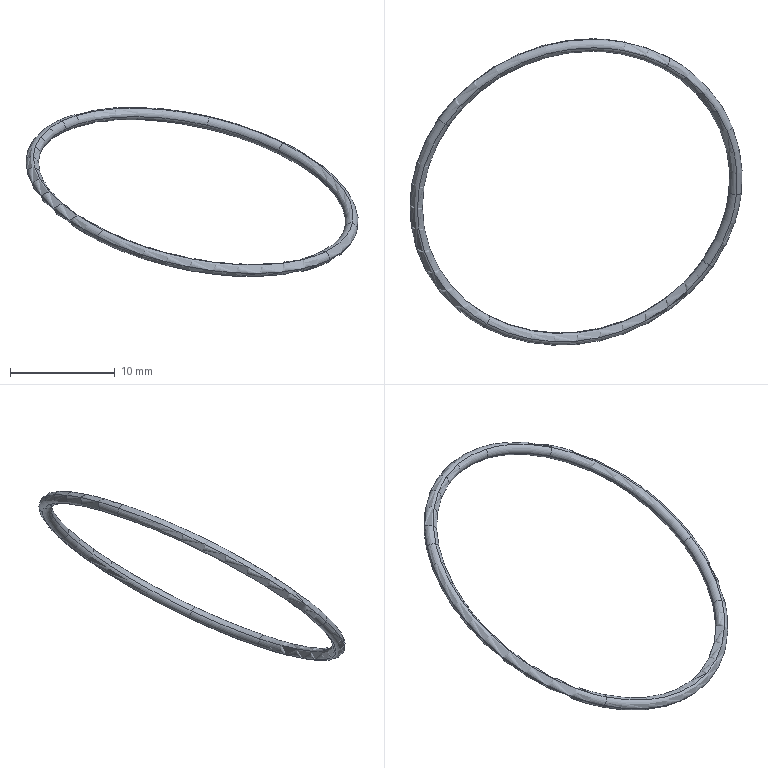Part | SolidWorks | features BaseBody 1 | 1 solid | 22 faces | box 31.731 x 29.251 x 16.171 mm | volume 110.749 mm3 | torus 22
STEP:
#1=CARTESIAN_POINT('',(1961.202,-199.266,900.389));
#2=VERTEX_POINT('',#1);
#3=CARTESIAN_POINT('',(1954.63,-186.958,908.017));
#4=VERTEX_POINT('',#3);
#5=CARTESIAN_POINT('',(1961.202,-199.266,900.389));
#6=CARTESIAN_POINT('',(1961.789,-193.856,902.943));
#7=CARTESIAN_POINT('',(1959.22,-189.407,905.745));
#8=CARTESIAN_POINT('',(1954.63,-186.958,908.017));
#9=(BOUNDED_CURVE()B_SPLINE_CURVE(3,(#5,#6,#7,#8),.UNSPECIFIED.,.F.,.F.)B_SPLINE_CURVE_WITH_KNOTS((4,4),(0.3237,1.),.UNSPECIFIED.)CURVE()GEOMETRIC_REPRESENTATION_ITEM()RATIONAL_B_SPLINE_CURVE((1.167,1.112,1.178,1.363))REPRESENTATION_ITEM(''));
#10=EDGE_CURVE('',#2,#4,#9,.T.);
#11=ORIENTED_EDGE('',*,*,#10,.F.);
#12=CARTESIAN_POINT('',(1960.738,-199.528,901.049));
#13=VERTEX_POINT('',#12);
#14=CARTESIAN_POINT('',(1961.323,-199.528,900.915));
#15=DIRECTION('',(0.09761,0.8999,0.425));
#16=DIRECTION('',(0.,-0.427,0.9043));
#17=AXIS2_PLACEMENT_3D('',#14,#15,#16);
#18=CIRCLE('',#17,0.6);
#19=EDGE_CURVE('',#2,#13,#18,.T.);
#20=ORIENTED_EDGE('',*,*,#19,.T.);
#21=CARTESIAN_POINT('',(1954.419,-187.693,908.384));
#22=VERTEX_POINT('',#21);
#23=CARTESIAN_POINT('',(1960.738,-199.528,901.049));
#24=CARTESIAN_POINT('',(1961.302,-194.326,903.505));
#25=CARTESIAN_POINT('',(1958.832,-190.049,906.199));
#26=CARTESIAN_POINT('',(1954.419,-187.693,908.384));
#27=(BOUNDED_CURVE()B_SPLINE_CURVE(3,(#23,#24,#25,#26),.UNSPECIFIED.,.F.,.F.)B_SPLINE_CURVE_WITH_KNOTS((4,4),(0.3237,1.),.UNSPECIFIED.)CURVE()GEOMETRIC_REPRESENTATION_ITEM()RATIONAL_B_SPLINE_CURVE((1.216,1.159,1.228,1.421))REPRESENTATION_ITEM(''));
#28=EDGE_CURVE('',#13,#22,#27,.T.);
#29=ORIENTED_EDGE('',*,*,#28,.T.);
#30=CARTESIAN_POINT('',(1954.63,-186.958,908.017));
#31=CARTESIAN_POINT('',(1954.434,-187.238,907.923));
#32=CARTESIAN_POINT('',(1954.349,-187.541,908.078));
#33=CARTESIAN_POINT('',(1954.419,-187.693,908.384));
#34=(BOUNDED_CURVE()B_SPLINE_CURVE(3,(#30,#31,#32,#33),.UNSPECIFIED.,.F.,.T.)B_SPLINE_CURVE_WITH_KNOTS((4,4),(0.,1.),.UNSPECIFIED.)CURVE()GEOMETRIC_REPRESENTATION_ITEM()RATIONAL_B_SPLINE_CURVE((1.363,1.111,1.13,1.421))REPRESENTATION_ITEM(''));
#35=EDGE_CURVE('',#4,#22,#34,.T.);
#36=ORIENTED_EDGE('',*,*,#35,.F.);
#37=EDGE_LOOP('',(#11,#20,#29,#36));
#38=FACE_OUTER_BOUND('',#37,.T.);
#39=CARTESIAN_POINT('',(1946.133,-199.528,904.404));
#40=DIRECTION('',(-0.2015,0.436,-0.8771));
#41=DIRECTION('',(0.9746,0.,-0.2239));
#42=AXIS2_PLACEMENT_3D('',#39,#40,#41);
#43=TOROIDAL_SURFACE('',#42,15.585,0.6);
#44=ADVANCED_FACE('',(#38),#43,.T.);
#45=CARTESIAN_POINT('',(1947.596,-186.042,910.772));
#46=VERTEX_POINT('',#45);
#47=CARTESIAN_POINT('',(1934.018,-193.063,910.401));
#48=VERTEX_POINT('',#47);
#49=CARTESIAN_POINT('',(1947.596,-186.042,910.772));
#50=CARTESIAN_POINT('',(1941.997,-186.042,912.058));
#51=CARTESIAN_POINT('',(1937.057,-188.722,911.86));
#52=CARTESIAN_POINT('',(1934.018,-193.063,910.401));
#53=(BOUNDED_CURVE()B_SPLINE_CURVE(3,(#49,#50,#51,#52),.UNSPECIFIED.,.F.,.T.)B_SPLINE_CURVE_WITH_KNOTS((4,4),(0.3294,1.),.UNSPECIFIED.)CURVE()GEOMETRIC_REPRESENTATION_ITEM()RATIONAL_B_SPLINE_CURVE((1.228,1.157,1.209,1.385))REPRESENTATION_ITEM(''));
#54=EDGE_CURVE('',#46,#48,#53,.T.);
#55=ORIENTED_EDGE('',*,*,#54,.F.);
#56=CARTESIAN_POINT('',(1947.776,-185.764,911.553));
#57=VERTEX_POINT('',#56);
#58=CARTESIAN_POINT('',(1947.655,-185.502,911.027));
#59=DIRECTION('',(-0.9746,0.,0.2239));
#60=DIRECTION('',(0.2239,0.,0.9746));
#61=AXIS2_PLACEMENT_3D('',#58,#59,#60);
#62=CIRCLE('',#61,0.6);
#63=EDGE_CURVE('',#46,#57,#62,.T.);
#64=ORIENTED_EDGE('',*,*,#63,.T.);
#65=CARTESIAN_POINT('',(1933.654,-193.065,911.167));
#66=VERTEX_POINT('',#65);
#67=CARTESIAN_POINT('',(1947.776,-185.764,911.553));
#68=CARTESIAN_POINT('',(1941.953,-185.764,912.89));
#69=CARTESIAN_POINT('',(1936.814,-188.551,912.685));
#70=CARTESIAN_POINT('',(1933.654,-193.065,911.167));
#71=(BOUNDED_CURVE()B_SPLINE_CURVE(3,(#67,#68,#69,#70),.UNSPECIFIED.,.F.,.F.)B_SPLINE_CURVE_WITH_KNOTS((4,4),(0.3294,1.),.UNSPECIFIED.)CURVE()GEOMETRIC_REPRESENTATION_ITEM()RATIONAL_B_SPLINE_CURVE((1.178,1.11,1.16,1.328))REPRESENTATION_ITEM(''));
#72=EDGE_CURVE('',#57,#66,#71,.T.);
#73=ORIENTED_EDGE('',*,*,#72,.T.);
#74=CARTESIAN_POINT('',(1934.018,-193.063,910.401));
#75=CARTESIAN_POINT('',(1934.088,-193.215,910.706));
#76=CARTESIAN_POINT('',(1933.94,-193.218,911.025));
#77=CARTESIAN_POINT('',(1933.654,-193.065,911.167));
#78=(BOUNDED_CURVE()B_SPLINE_CURVE(3,(#74,#75,#76,#77),.UNSPECIFIED.,.F.,.F.)B_SPLINE_CURVE_WITH_KNOTS((4,4),(0.,1.),.UNSPECIFIED.)CURVE()GEOMETRIC_REPRESENTATION_ITEM()RATIONAL_B_SPLINE_CURVE((1.385,1.101,1.082,1.328))REPRESENTATION_ITEM(''));
#79=EDGE_CURVE('',#48,#66,#78,.T.);
#80=ORIENTED_EDGE('',*,*,#79,.F.);
#81=EDGE_LOOP('',(#55,#64,#73,#80));
#82=FACE_OUTER_BOUND('',#81,.T.);
#83=CARTESIAN_POINT('',(1946.133,-199.528,904.404));
#84=DIRECTION('',(-0.2015,0.436,-0.8771));
#85=DIRECTION('',(0.09761,0.8999,0.425));
#86=AXIS2_PLACEMENT_3D('',#83,#84,#85);
#87=TOROIDAL_SURFACE('',#86,15.585,0.6);
#88=ADVANCED_FACE('',(#82),#87,.T.);
#89=CARTESIAN_POINT('',(1947.713,-184.963,911.282));
#90=VERTEX_POINT('',#89);
#91=CARTESIAN_POINT('',(1933.048,-192.545,910.881));
#92=VERTEX_POINT('',#91);
#93=CARTESIAN_POINT('',(1947.713,-184.963,911.282));
#94=CARTESIAN_POINT('',(1941.666,-184.963,912.671));
#95=CARTESIAN_POINT('',(1936.33,-187.857,912.457));
#96=CARTESIAN_POINT('',(1933.048,-192.545,910.881));
#97=(BOUNDED_CURVE()B_SPLINE_CURVE(3,(#93,#94,#95,#96),.UNSPECIFIED.,.F.,.F.)B_SPLINE_CURVE_WITH_KNOTS((4,4),(0.3294,1.),.UNSPECIFIED.)CURVE()GEOMETRIC_REPRESENTATION_ITEM()RATIONAL_B_SPLINE_CURVE((1.228,1.157,1.209,1.385))REPRESENTATION_ITEM(''));
#98=EDGE_CURVE('',#90,#92,#97,.T.);
#99=ORIENTED_EDGE('',*,*,#98,.F.);
#100=CARTESIAN_POINT('',(1947.534,-185.241,910.5));
#101=VERTEX_POINT('',#100);
#102=CARTESIAN_POINT('',(1947.655,-185.502,911.027));
#103=DIRECTION('',(-0.9746,0.,0.2239));
#104=DIRECTION('',(0.2239,0.,0.9746));
#105=AXIS2_PLACEMENT_3D('',#102,#103,#104);
#106=CIRCLE('',#105,0.6);
#107=EDGE_CURVE('',#90,#101,#106,.T.);
#108=ORIENTED_EDGE('',*,*,#107,.T.);
#109=CARTESIAN_POINT('',(1933.412,-192.542,910.115));
#110=VERTEX_POINT('',#109);
#111=CARTESIAN_POINT('',(1947.534,-185.241,910.5));
#112=CARTESIAN_POINT('',(1941.711,-185.241,911.838));
#113=CARTESIAN_POINT('',(1936.572,-188.028,911.633));
#114=CARTESIAN_POINT('',(1933.412,-192.542,910.115));
#115=(BOUNDED_CURVE()B_SPLINE_CURVE(3,(#111,#112,#113,#114),.UNSPECIFIED.,.F.,.F.)B_SPLINE_CURVE_WITH_KNOTS((4,4),(0.3294,1.),.UNSPECIFIED.)CURVE()GEOMETRIC_REPRESENTATION_ITEM()RATIONAL_B_SPLINE_CURVE((1.178,1.11,1.16,1.328))REPRESENTATION_ITEM(''));
#116=EDGE_CURVE('',#101,#110,#115,.T.);
#117=ORIENTED_EDGE('',*,*,#116,.T.);
#118=CARTESIAN_POINT('',(1933.048,-192.545,910.881));
#119=CARTESIAN_POINT('',(1932.977,-192.393,910.575));
#120=CARTESIAN_POINT('',(1933.125,-192.389,910.256));
#121=CARTESIAN_POINT('',(1933.412,-192.542,910.115));
#122=(BOUNDED_CURVE()B_SPLINE_CURVE(3,(#118,#119,#120,#121),.UNSPECIFIED.,.F.,.F.)B_SPLINE_CURVE_WITH_KNOTS((4,4),(0.,1.),.UNSPECIFIED.)CURVE()GEOMETRIC_REPRESENTATION_ITEM()RATIONAL_B_SPLINE_CURVE((1.385,1.101,1.082,1.328))REPRESENTATION_ITEM(''));
#123=EDGE_CURVE('',#92,#110,#122,.T.);
#124=ORIENTED_EDGE('',*,*,#123,.F.);
#125=EDGE_LOOP('',(#99,#108,#117,#124));
#126=FACE_OUTER_BOUND('',#125,.T.);
#127=CARTESIAN_POINT('',(1946.133,-199.528,904.404));
#128=DIRECTION('',(-0.2015,0.436,-0.8771));
#129=DIRECTION('',(0.09761,0.8999,0.425));
#130=AXIS2_PLACEMENT_3D('',#127,#128,#129);
#131=TOROIDAL_SURFACE('',#130,15.585,0.6);
#132=ADVANCED_FACE('',(#126),#131,.T.);
#133=ORIENTED_EDGE('',*,*,#28,.F.);
#134=CARTESIAN_POINT('',(1961.444,-199.79,901.441));
#135=VERTEX_POINT('',#134);
#136=CARTESIAN_POINT('',(1961.323,-199.528,900.915));
#137=DIRECTION('',(0.09761,0.8999,0.425));
#138=DIRECTION('',(0.,-0.427,0.9043));
#139=AXIS2_PLACEMENT_3D('',#136,#137,#138);
#140=CIRCLE('',#139,0.6);
#141=EDGE_CURVE('',#13,#135,#140,.T.);
#142=ORIENTED_EDGE('',*,*,#141,.T.);
#143=CARTESIAN_POINT('',(1954.871,-187.481,909.069));
#144=VERTEX_POINT('',#143);
#145=CARTESIAN_POINT('',(1961.444,-199.79,901.441));
#146=CARTESIAN_POINT('',(1962.03,-194.38,903.996));
#147=CARTESIAN_POINT('',(1959.462,-189.931,906.797));
#148=CARTESIAN_POINT('',(1954.871,-187.481,909.069));
#149=(BOUNDED_CURVE()B_SPLINE_CURVE(3,(#145,#146,#147,#148),.UNSPECIFIED.,.F.,.F.)B_SPLINE_CURVE_WITH_KNOTS((4,4),(0.3237,1.),.UNSPECIFIED.)CURVE()GEOMETRIC_REPRESENTATION_ITEM()RATIONAL_B_SPLINE_CURVE((1.167,1.112,1.178,1.363))REPRESENTATION_ITEM(''));
#150=EDGE_CURVE('',#135,#144,#149,.T.);
#151=ORIENTED_EDGE('',*,*,#150,.T.);
#152=CARTESIAN_POINT('',(1954.419,-187.693,908.384));
#153=CARTESIAN_POINT('',(1954.489,-187.845,908.689));
#154=CARTESIAN_POINT('',(1954.675,-187.761,908.975));
#155=CARTESIAN_POINT('',(1954.871,-187.481,909.069));
#156=(BOUNDED_CURVE()B_SPLINE_CURVE(3,(#152,#153,#154,#155),.UNSPECIFIED.,.F.,.F.)B_SPLINE_CURVE_WITH_KNOTS((4,4),(0.,1.),.UNSPECIFIED.)CURVE()GEOMETRIC_REPRESENTATION_ITEM()RATIONAL_B_SPLINE_CURVE((1.421,1.13,1.111,1.363))REPRESENTATION_ITEM(''));
#157=EDGE_CURVE('',#22,#144,#156,.T.);
#158=ORIENTED_EDGE('',*,*,#157,.F.);
#159=EDGE_LOOP('',(#133,#142,#151,#158));
#160=FACE_OUTER_BOUND('',#159,.T.);
#161=CARTESIAN_POINT('',(1946.133,-199.528,904.404));
#162=DIRECTION('',(-0.2015,0.436,-0.8771));
#163=DIRECTION('',(0.9746,0.,-0.2239));
#164=AXIS2_PLACEMENT_3D('',#161,#162,#163);
#165=TOROIDAL_SURFACE('',#164,15.585,0.6);
#166=ADVANCED_FACE('',(#160),#165,.T.);
#167=CARTESIAN_POINT('',(1961.908,-199.528,900.78));
#168=VERTEX_POINT('',#167);
#169=CARTESIAN_POINT('',(1955.082,-186.746,908.702));
#170=VERTEX_POINT('',#169);
#171=CARTESIAN_POINT('',(1961.908,-199.528,900.78));
#172=CARTESIAN_POINT('',(1962.517,-193.91,903.433));
#173=CARTESIAN_POINT('',(1959.849,-189.289,906.343));
#174=CARTESIAN_POINT('',(1955.082,-186.746,908.702));
#175=(BOUNDED_CURVE()B_SPLINE_CURVE(3,(#171,#172,#173,#174),.UNSPECIFIED.,.F.,.F.)B_SPLINE_CURVE_WITH_KNOTS((4,4),(0.3237,1.),.UNSPECIFIED.)CURVE()GEOMETRIC_REPRESENTATION_ITEM()RATIONAL_B_SPLINE_CURVE((1.216,1.159,1.228,1.421))REPRESENTATION_ITEM(''));
#176=EDGE_CURVE('',#168,#170,#175,.T.);
#177=ORIENTED_EDGE('',*,*,#176,.F.);
#178=CARTESIAN_POINT('',(1961.323,-199.528,900.915));
#179=DIRECTION('',(0.09761,0.8999,0.425));
#180=DIRECTION('',(0.,-0.427,0.9043));
#181=AXIS2_PLACEMENT_3D('',#178,#179,#180);
#182=CIRCLE('',#181,0.6);
#183=EDGE_CURVE('',#168,#2,#182,.T.);
#184=ORIENTED_EDGE('',*,*,#183,.T.);
#185=ORIENTED_EDGE('',*,*,#10,.T.);
#186=CARTESIAN_POINT('',(1955.082,-186.746,908.702));
#187=CARTESIAN_POINT('',(1955.012,-186.594,908.397));
#188=CARTESIAN_POINT('',(1954.826,-186.678,908.111));
#189=CARTESIAN_POINT('',(1954.63,-186.958,908.017));
#190=(BOUNDED_CURVE()B_SPLINE_CURVE(3,(#186,#187,#188,#189),.UNSPECIFIED.,.F.,.F.)B_SPLINE_CURVE_WITH_KNOTS((4,4),(0.,1.),.UNSPECIFIED.)CURVE()GEOMETRIC_REPRESENTATION_ITEM()RATIONAL_B_SPLINE_CURVE((1.421,1.13,1.111,1.363))REPRESENTATION_ITEM(''));
#191=EDGE_CURVE('',#170,#4,#190,.T.);
#192=ORIENTED_EDGE('',*,*,#191,.F.);
#193=EDGE_LOOP('',(#177,#184,#185,#192));
#194=FACE_OUTER_BOUND('',#193,.T.);
#195=CARTESIAN_POINT('',(1946.133,-199.528,904.404));
#196=DIRECTION('',(-0.2015,0.436,-0.8771));
#197=DIRECTION('',(0.9746,0.,-0.2239));
#198=AXIS2_PLACEMENT_3D('',#195,#196,#197);
#199=TOROIDAL_SURFACE('',#198,15.585,0.6);
#200=ADVANCED_FACE('',(#194),#199,.T.);
#201=ORIENTED_EDGE('',*,*,#150,.F.);
#202=CARTESIAN_POINT('',(1961.323,-199.528,900.915));
#203=DIRECTION('',(0.09761,0.8999,0.425));
#204=DIRECTION('',(0.,-0.427,0.9043));
#205=AXIS2_PLACEMENT_3D('',#202,#203,#204);
#206=CIRCLE('',#205,0.6);
#207=EDGE_CURVE('',#135,#168,#206,.T.);
#208=ORIENTED_EDGE('',*,*,#207,.T.);
#209=ORIENTED_EDGE('',*,*,#176,.T.);
#210=CARTESIAN_POINT('',(1954.871,-187.481,909.069));
#211=CARTESIAN_POINT('',(1955.067,-187.201,909.164));
#212=CARTESIAN_POINT('',(1955.153,-186.898,909.008));
#213=CARTESIAN_POINT('',(1955.082,-186.746,908.702));
#214=(BOUNDED_CURVE()B_SPLINE_CURVE(3,(#210,#211,#212,#213),.UNSPECIFIED.,.F.,.F.)B_SPLINE_CURVE_WITH_KNOTS((4,4),(0.,1.),.UNSPECIFIED.)CURVE()GEOMETRIC_REPRESENTATION_ITEM()RATIONAL_B_SPLINE_CURVE((1.363,1.111,1.13,1.421))REPRESENTATION_ITEM(''));
#215=EDGE_CURVE('',#144,#170,#214,.T.);
#216=ORIENTED_EDGE('',*,*,#215,.F.);
#217=EDGE_LOOP('',(#201,#208,#209,#216));
#218=FACE_OUTER_BOUND('',#217,.T.);
#219=CARTESIAN_POINT('',(1946.133,-199.528,904.404));
#220=DIRECTION('',(-0.2015,0.436,-0.8771));
#221=DIRECTION('',(0.9746,0.,-0.2239));
#222=AXIS2_PLACEMENT_3D('',#219,#220,#221);
#223=TOROIDAL_SURFACE('',#222,15.585,0.6);
#224=ADVANCED_FACE('',(#218),#223,.T.);
#225=CARTESIAN_POINT('',(1937.637,-212.098,900.791));
#226=VERTEX_POINT('',#225);
#227=CARTESIAN_POINT('',(1937.184,-212.31,900.105));
#228=VERTEX_POINT('',#227);
#229=CARTESIAN_POINT('',(1937.637,-212.098,900.791));
#230=CARTESIAN_POINT('',(1937.441,-212.378,900.696));
#231=CARTESIAN_POINT('',(1937.255,-212.462,900.411));
#232=CARTESIAN_POINT('',(1937.184,-212.31,900.105));
#233=(BOUNDED_CURVE()B_SPLINE_CURVE(3,(#229,#230,#231,#232),.UNSPECIFIED.,.F.,.F.)B_SPLINE_CURVE_WITH_KNOTS((4,4),(0.,1.),.UNSPECIFIED.)CURVE()GEOMETRIC_REPRESENTATION_ITEM()RATIONAL_B_SPLINE_CURVE((1.363,1.111,1.13,1.421))REPRESENTATION_ITEM(''));
#234=EDGE_CURVE('',#226,#228,#233,.T.);
#235=ORIENTED_EDGE('',*,*,#234,.T.);
#236=CARTESIAN_POINT('',(1959.219,-206.511,897.927));
#237=VERTEX_POINT('',#236);
#238=CARTESIAN_POINT('',(1937.184,-212.31,900.105));
#239=CARTESIAN_POINT('',(1944.808,-216.379,896.331));
#240=CARTESIAN_POINT('',(1953.949,-214.039,895.395));
#241=CARTESIAN_POINT('',(1959.219,-206.511,897.927));
#242=(BOUNDED_CURVE()B_SPLINE_CURVE(3,(#238,#239,#240,#241),.UNSPECIFIED.,.F.,.F.)B_SPLINE_CURVE_WITH_KNOTS((4,4),(0.,1.),.UNSPECIFIED.)CURVE()GEOMETRIC_REPRESENTATION_ITEM()RATIONAL_B_SPLINE_CURVE((1.421,1.135,1.123,1.385))REPRESENTATION_ITEM(''));
#243=EDGE_CURVE('',#228,#237,#242,.T.);
#244=ORIENTED_EDGE('',*,*,#243,.T.);
#245=CARTESIAN_POINT('',(1958.855,-206.514,898.693));
#246=VERTEX_POINT('',#245);
#247=CARTESIAN_POINT('',(1958.734,-206.252,898.167));
#248=DIRECTION('',(0.5529,0.7898,0.2656));
#249=DIRECTION('',(0.8085,-0.4315,-0.4002));
#250=AXIS2_PLACEMENT_3D('',#247,#248,#249);
#251=CIRCLE('',#250,0.6);
#252=EDGE_CURVE('',#246,#237,#251,.T.);
#253=ORIENTED_EDGE('',*,*,#252,.F.);
#254=CARTESIAN_POINT('',(1937.637,-212.098,900.791));
#255=CARTESIAN_POINT('',(1944.978,-216.016,897.157));
#256=CARTESIAN_POINT('',(1953.78,-213.763,896.255));
#257=CARTESIAN_POINT('',(1958.855,-206.514,898.693));
#258=(BOUNDED_CURVE()B_SPLINE_CURVE(3,(#254,#255,#256,#257),.UNSPECIFIED.,.F.,.F.)B_SPLINE_CURVE_WITH_KNOTS((4,4),(0.,1.),.UNSPECIFIED.)CURVE()GEOMETRIC_REPRESENTATION_ITEM()RATIONAL_B_SPLINE_CURVE((1.363,1.089,1.077,1.328))REPRESENTATION_ITEM(''));
#259=EDGE_CURVE('',#226,#246,#258,.T.);
#260=ORIENTED_EDGE('',*,*,#259,.F.);
#261=EDGE_LOOP('',(#235,#244,#253,#260));
#262=FACE_OUTER_BOUND('',#261,.T.);
#263=CARTESIAN_POINT('',(1946.133,-199.528,904.404));
#264=DIRECTION('',(-0.2015,0.436,-0.8771));
#265=DIRECTION('',(0.9746,0.,-0.2239));
#266=AXIS2_PLACEMENT_3D('',#263,#264,#265);
#267=TOROIDAL_SURFACE('',#266,15.585,0.6);
#268=ADVANCED_FACE('',(#262),#267,.T.);
#269=CARTESIAN_POINT('',(1933.048,-192.545,910.881));
#270=CARTESIAN_POINT('',(1927.777,-200.073,908.349));
#271=CARTESIAN_POINT('',(1929.56,-208.242,903.879));
#272=CARTESIAN_POINT('',(1937.184,-212.31,900.105));
#273=(BOUNDED_CURVE()B_SPLINE_CURVE(3,(#269,#270,#271,#272),.UNSPECIFIED.,.F.,.F.)B_SPLINE_CURVE_WITH_KNOTS((4,4),(0.,1.),.UNSPECIFIED.)CURVE()GEOMETRIC_REPRESENTATION_ITEM()RATIONAL_B_SPLINE_CURVE((1.385,1.123,1.135,1.421))REPRESENTATION_ITEM(''));
#274=EDGE_CURVE('',#92,#228,#273,.T.);
#275=ORIENTED_EDGE('',*,*,#274,.T.);
#276=ORIENTED_EDGE('',*,*,#234,.F.);
#277=CARTESIAN_POINT('',(1933.654,-193.065,911.167));
#278=CARTESIAN_POINT('',(1928.579,-200.314,908.729));
#279=CARTESIAN_POINT('',(1930.296,-208.181,904.424));
#280=CARTESIAN_POINT('',(1937.637,-212.098,900.791));
#281=(BOUNDED_CURVE()B_SPLINE_CURVE(3,(#277,#278,#279,#280),.UNSPECIFIED.,.F.,.T.)B_SPLINE_CURVE_WITH_KNOTS((4,4),(0.,1.),.UNSPECIFIED.)CURVE()GEOMETRIC_REPRESENTATION_ITEM()RATIONAL_B_SPLINE_CURVE((1.328,1.077,1.089,1.363))REPRESENTATION_ITEM(''));
#282=EDGE_CURVE('',#66,#226,#281,.T.);
#283=ORIENTED_EDGE('',*,*,#282,.F.);
#284=CARTESIAN_POINT('',(1933.654,-193.065,911.167));
#285=CARTESIAN_POINT('',(1933.367,-192.912,911.309));
#286=CARTESIAN_POINT('',(1933.118,-192.697,911.187));
#287=CARTESIAN_POINT('',(1933.048,-192.545,910.881));
#288=(BOUNDED_CURVE()B_SPLINE_CURVE(3,(#284,#285,#286,#287),.UNSPECIFIED.,.F.,.T.)B_SPLINE_CURVE_WITH_KNOTS((4,4),(0.,1.),.UNSPECIFIED.)CURVE()GEOMETRIC_REPRESENTATION_ITEM()RATIONAL_B_SPLINE_CURVE((1.328,1.082,1.101,1.385))REPRESENTATION_ITEM(''));
#289=EDGE_CURVE('',#66,#92,#288,.T.);
#290=ORIENTED_EDGE('',*,*,#289,.T.);
#291=EDGE_LOOP('',(#275,#276,#283,#290));
#292=FACE_OUTER_BOUND('',#291,.T.);
#293=CARTESIAN_POINT('',(1946.133,-199.528,904.404));
#294=DIRECTION('',(-0.2015,0.436,-0.8771));
#295=DIRECTION('',(0.9746,0.,-0.2239));
#296=AXIS2_PLACEMENT_3D('',#293,#294,#295);
#297=TOROIDAL_SURFACE('',#296,15.585,0.6);
#298=ADVANCED_FACE('',(#292),#297,.T.);
#299=ORIENTED_EDGE('',*,*,#243,.F.);
#300=CARTESIAN_POINT('',(1937.395,-211.575,899.738));
#301=VERTEX_POINT('',#300);
#302=CARTESIAN_POINT('',(1937.184,-212.31,900.105));
#303=CARTESIAN_POINT('',(1937.114,-212.159,899.799));
#304=CARTESIAN_POINT('',(1937.199,-211.855,899.644));
#305=CARTESIAN_POINT('',(1937.395,-211.575,899.738));
#306=(BOUNDED_CURVE()B_SPLINE_CURVE(3,(#302,#303,#304,#305),.UNSPECIFIED.,.F.,.F.)B_SPLINE_CURVE_WITH_KNOTS((4,4),(0.,1.),.UNSPECIFIED.)CURVE()GEOMETRIC_REPRESENTATION_ITEM()RATIONAL_B_SPLINE_CURVE((1.421,1.13,1.111,1.363))REPRESENTATION_ITEM(''));
#307=EDGE_CURVE('',#228,#301,#306,.T.);
#308=ORIENTED_EDGE('',*,*,#307,.T.);
#309=CARTESIAN_POINT('',(1958.613,-205.991,897.64));
#310=VERTEX_POINT('',#309);
#311=CARTESIAN_POINT('',(1937.395,-211.575,899.738));
#312=CARTESIAN_POINT('',(1944.737,-215.493,896.104));
#313=CARTESIAN_POINT('',(1953.538,-213.24,895.203));
#314=CARTESIAN_POINT('',(1958.613,-205.991,897.64));
#315=(BOUNDED_CURVE()B_SPLINE_CURVE(3,(#311,#312,#313,#314),.UNSPECIFIED.,.F.,.F.)B_SPLINE_CURVE_WITH_KNOTS((4,4),(0.,1.),.UNSPECIFIED.)CURVE()GEOMETRIC_REPRESENTATION_ITEM()RATIONAL_B_SPLINE_CURVE((1.363,1.089,1.077,1.328))REPRESENTATION_ITEM(''));
#316=EDGE_CURVE('',#301,#310,#315,.T.);
#317=ORIENTED_EDGE('',*,*,#316,.T.);
#318=CARTESIAN_POINT('',(1959.219,-206.511,897.927));
#319=CARTESIAN_POINT('',(1959.149,-206.359,897.621));
#320=CARTESIAN_POINT('',(1958.9,-206.144,897.499));
#321=CARTESIAN_POINT('',(1958.613,-205.991,897.64));
#322=(BOUNDED_CURVE()B_SPLINE_CURVE(3,(#318,#319,#320,#321),.UNSPECIFIED.,.F.,.F.)B_SPLINE_CURVE_WITH_KNOTS((4,4),(0.,1.),.UNSPECIFIED.)CURVE()GEOMETRIC_REPRESENTATION_ITEM()RATIONAL_B_SPLINE_CURVE((1.385,1.101,1.082,1.328))REPRESENTATION_ITEM(''));
#323=EDGE_CURVE('',#237,#310,#322,.T.);
#324=ORIENTED_EDGE('',*,*,#323,.F.);
#325=EDGE_LOOP('',(#299,#308,#317,#324));
#326=FACE_OUTER_BOUND('',#325,.T.);
#327=CARTESIAN_POINT('',(1946.133,-199.528,904.404));
#328=DIRECTION('',(-0.2015,0.436,-0.8771));
#329=DIRECTION('',(0.09761,0.8999,0.425));
#330=AXIS2_PLACEMENT_3D('',#327,#328,#329);
#331=TOROIDAL_SURFACE('',#330,15.585,0.6);
#332=ADVANCED_FACE('',(#326),#331,.T.);
#333=ORIENTED_EDGE('',*,*,#207,.F.);
#334=CARTESIAN_POINT('',(1958.855,-206.514,898.693));
#335=CARTESIAN_POINT('',(1960.274,-204.487,899.375));
#336=CARTESIAN_POINT('',(1961.182,-202.203,900.301));
#337=CARTESIAN_POINT('',(1961.444,-199.79,901.441));
#338=(BOUNDED_CURVE()B_SPLINE_CURVE(3,(#334,#335,#336,#337),.UNSPECIFIED.,.F.,.F.)B_SPLINE_CURVE_WITH_KNOTS((4,4),(0.,0.3237),.UNSPECIFIED.)CURVE()GEOMETRIC_REPRESENTATION_ITEM()RATIONAL_B_SPLINE_CURVE((1.328,1.247,1.193,1.167))REPRESENTATION_ITEM(''));
#339=EDGE_CURVE('',#246,#135,#338,.T.);
#340=ORIENTED_EDGE('',*,*,#339,.F.);
#341=ORIENTED_EDGE('',*,*,#252,.T.);
#342=CARTESIAN_POINT('',(1959.219,-206.511,897.927));
#343=CARTESIAN_POINT('',(1960.693,-204.406,898.635));
#344=CARTESIAN_POINT('',(1961.636,-202.035,899.597));
#345=CARTESIAN_POINT('',(1961.908,-199.528,900.78));
#346=(BOUNDED_CURVE()B_SPLINE_CURVE(3,(#342,#343,#344,#345),.UNSPECIFIED.,.F.,.F.)B_SPLINE_CURVE_WITH_KNOTS((4,4),(0.,0.3237),.UNSPECIFIED.)CURVE()GEOMETRIC_REPRESENTATION_ITEM()RATIONAL_B_SPLINE_CURVE((1.385,1.3,1.244,1.216))REPRESENTATION_ITEM(''));
#347=EDGE_CURVE('',#237,#168,#346,.T.);
#348=ORIENTED_EDGE('',*,*,#347,.T.);
#349=EDGE_LOOP('',(#333,#340,#341,#348));
#350=FACE_OUTER_BOUND('',#349,.T.);
#351=CARTESIAN_POINT('',(1946.133,-199.528,904.404));
#352=DIRECTION('',(-0.2015,0.436,-0.8771));
#353=DIRECTION('',(0.9746,0.,-0.2239));
#354=AXIS2_PLACEMENT_3D('',#351,#352,#353);
#355=TOROIDAL_SURFACE('',#354,15.585,0.6);
#356=ADVANCED_FACE('',(#350),#355,.T.);
#357=CARTESIAN_POINT('',(1937.848,-211.363,900.424));
#358=VERTEX_POINT('',#357);
#359=CARTESIAN_POINT('',(1958.249,-205.993,898.407));
#360=VERTEX_POINT('',#359);
#361=CARTESIAN_POINT('',(1937.848,-211.363,900.424));
#362=CARTESIAN_POINT('',(1944.907,-215.13,896.93));
#363=CARTESIAN_POINT('',(1953.369,-212.963,896.063));
#364=CARTESIAN_POINT('',(1958.249,-205.993,898.407));
#365=(BOUNDED_CURVE()B_SPLINE_CURVE(3,(#361,#362,#363,#364),.UNSPECIFIED.,.F.,.F.)B_SPLINE_CURVE_WITH_KNOTS((4,4),(0.,1.),.UNSPECIFIED.)CURVE()GEOMETRIC_REPRESENTATION_ITEM()RATIONAL_B_SPLINE_CURVE((1.421,1.135,1.123,1.385))REPRESENTATION_ITEM(''));
#366=EDGE_CURVE('',#358,#360,#365,.T.);
#367=ORIENTED_EDGE('',*,*,#366,.F.);
#368=CARTESIAN_POINT('',(1937.848,-211.363,900.424));
#369=CARTESIAN_POINT('',(1937.918,-211.515,900.729));
#370=CARTESIAN_POINT('',(1937.833,-211.818,900.885));
#371=CARTESIAN_POINT('',(1937.637,-212.098,900.791));
#372=(BOUNDED_CURVE()B_SPLINE_CURVE(3,(#368,#369,#370,#371),.UNSPECIFIED.,.F.,.F.)B_SPLINE_CURVE_WITH_KNOTS((4,4),(0.,1.),.UNSPECIFIED.)CURVE()GEOMETRIC_REPRESENTATION_ITEM()RATIONAL_B_SPLINE_CURVE((1.421,1.13,1.111,1.363))REPRESENTATION_ITEM(''));
#373=EDGE_CURVE('',#358,#226,#372,.T.);
#374=ORIENTED_EDGE('',*,*,#373,.T.);
#375=ORIENTED_EDGE('',*,*,#259,.T.);
#376=CARTESIAN_POINT('',(1958.249,-205.993,898.407));
#377=CARTESIAN_POINT('',(1958.319,-206.145,898.712));
#378=CARTESIAN_POINT('',(1958.568,-206.361,898.835));
#379=CARTESIAN_POINT('',(1958.855,-206.514,898.693));
#380=(BOUNDED_CURVE()B_SPLINE_CURVE(3,(#376,#377,#378,#379),.UNSPECIFIED.,.F.,.F.)B_SPLINE_CURVE_WITH_KNOTS((4,4),(0.,1.),.UNSPECIFIED.)CURVE()GEOMETRIC_REPRESENTATION_ITEM()RATIONAL_B_SPLINE_CURVE((1.385,1.101,1.082,1.328))REPRESENTATION_ITEM(''));
#381=EDGE_CURVE('',#360,#246,#380,.T.);
#382=ORIENTED_EDGE('',*,*,#381,.F.);
#383=EDGE_LOOP('',(#367,#374,#375,#382));
#384=FACE_OUTER_BOUND('',#383,.T.);
#385=CARTESIAN_POINT('',(1946.133,-199.528,904.404));
#386=DIRECTION('',(-0.2015,0.436,-0.8771));
#387=DIRECTION('',(0.09761,0.8999,0.425));
#388=AXIS2_PLACEMENT_3D('',#385,#386,#387);
#389=TOROIDAL_SURFACE('',#388,15.585,0.6);
#390=ADVANCED_FACE('',(#384),#389,.T.);
#391=ORIENTED_EDGE('',*,*,#307,.F.);
#392=ORIENTED_EDGE('',*,*,#274,.F.);
#393=ORIENTED_EDGE('',*,*,#123,.T.);
#394=CARTESIAN_POINT('',(1933.412,-192.542,910.115));
#395=CARTESIAN_POINT('',(1928.337,-199.791,907.677));
#396=CARTESIAN_POINT('',(1930.054,-207.657,903.372));
#397=CARTESIAN_POINT('',(1937.395,-211.575,899.738));
#398=(BOUNDED_CURVE()B_SPLINE_CURVE(3,(#394,#395,#396,#397),.UNSPECIFIED.,.F.,.F.)B_SPLINE_CURVE_WITH_KNOTS((4,4),(0.,1.),.UNSPECIFIED.)CURVE()GEOMETRIC_REPRESENTATION_ITEM()RATIONAL_B_SPLINE_CURVE((1.328,1.077,1.089,1.363))REPRESENTATION_ITEM(''));
#399=EDGE_CURVE('',#110,#301,#398,.T.);
#400=ORIENTED_EDGE('',*,*,#399,.T.);
#401=EDGE_LOOP('',(#391,#392,#393,#400));
#402=FACE_OUTER_BOUND('',#401,.T.);
#403=CARTESIAN_POINT('',(1946.133,-199.528,904.404));
#404=DIRECTION('',(-0.2015,0.436,-0.8771));
#405=DIRECTION('',(0.9746,0.,-0.2239));
#406=AXIS2_PLACEMENT_3D('',#403,#404,#405);
#407=TOROIDAL_SURFACE('',#406,15.585,0.6);
#408=ADVANCED_FACE('',(#402),#407,.T.);
#409=ORIENTED_EDGE('',*,*,#373,.F.);
#410=CARTESIAN_POINT('',(1934.018,-193.063,910.401));
#411=CARTESIAN_POINT('',(1929.138,-200.033,908.057));
#412=CARTESIAN_POINT('',(1930.789,-207.596,903.918));
#413=CARTESIAN_POINT('',(1937.848,-211.363,900.424));
#414=(BOUNDED_CURVE()B_SPLINE_CURVE(3,(#410,#411,#412,#413),.UNSPECIFIED.,.F.,.F.)B_SPLINE_CURVE_WITH_KNOTS((4,4),(0.,1.),.UNSPECIFIED.)CURVE()GEOMETRIC_REPRESENTATION_ITEM()RATIONAL_B_SPLINE_CURVE((1.385,1.123,1.135,1.421))REPRESENTATION_ITEM(''));
#415=EDGE_CURVE('',#48,#358,#414,.T.);
#416=ORIENTED_EDGE('',*,*,#415,.F.);
#417=ORIENTED_EDGE('',*,*,#79,.T.);
#418=ORIENTED_EDGE('',*,*,#282,.T.);
#419=EDGE_LOOP('',(#409,#416,#417,#418));
#420=FACE_OUTER_BOUND('',#419,.T.);
#421=CARTESIAN_POINT('',(1946.133,-199.528,904.404));
#422=DIRECTION('',(-0.2015,0.436,-0.8771));
#423=DIRECTION('',(0.9746,0.,-0.2239));
#424=AXIS2_PLACEMENT_3D('',#421,#422,#423);
#425=TOROIDAL_SURFACE('',#424,15.585,0.6);
#426=ADVANCED_FACE('',(#420),#425,.T.);
#427=ORIENTED_EDGE('',*,*,#215,.T.);
#428=CARTESIAN_POINT('',(1955.082,-186.746,908.702));
#429=CARTESIAN_POINT('',(1952.934,-185.599,909.766));
#430=CARTESIAN_POINT('',(1950.435,-184.963,910.656));
#431=CARTESIAN_POINT('',(1947.713,-184.963,911.282));
#432=(BOUNDED_CURVE()B_SPLINE_CURVE(3,(#428,#429,#430,#431),.UNSPECIFIED.,.F.,.F.)B_SPLINE_CURVE_WITH_KNOTS((4,4),(0.,0.3294),.UNSPECIFIED.)CURVE()GEOMETRIC_REPRESENTATION_ITEM()RATIONAL_B_SPLINE_CURVE((1.421,1.327,1.262,1.228))REPRESENTATION_ITEM(''));
#433=EDGE_CURVE('',#170,#90,#432,.T.);
#434=ORIENTED_EDGE('',*,*,#433,.T.);
#435=ORIENTED_EDGE('',*,*,#98,.T.);
#436=ORIENTED_EDGE('',*,*,#289,.F.);
#437=ORIENTED_EDGE('',*,*,#72,.F.);
#438=CARTESIAN_POINT('',(1954.871,-187.481,909.069));
#439=CARTESIAN_POINT('',(1952.803,-186.377,910.093));
#440=CARTESIAN_POINT('',(1950.397,-185.764,910.951));
#441=CARTESIAN_POINT('',(1947.776,-185.764,911.553));
#442=(BOUNDED_CURVE()B_SPLINE_CURVE(3,(#438,#439,#440,#441),.UNSPECIFIED.,.F.,.F.)B_SPLINE_CURVE_WITH_KNOTS((4,4),(0.,0.3294),.UNSPECIFIED.)CURVE()GEOMETRIC_REPRESENTATION_ITEM()RATIONAL_B_SPLINE_CURVE((1.363,1.273,1.211,1.178))REPRESENTATION_ITEM(''));
#443=EDGE_CURVE('',#144,#57,#442,.T.);
#444=ORIENTED_EDGE('',*,*,#443,.F.);
#445=EDGE_LOOP('',(#427,#434,#435,#436,#437,#444));
#446=FACE_OUTER_BOUND('',#445,.T.);
#447=CARTESIAN_POINT('',(1946.133,-199.528,904.404));
#448=DIRECTION('',(-0.2015,0.436,-0.8771));
#449=DIRECTION('',(0.9746,0.,-0.2239));
#450=AXIS2_PLACEMENT_3D('',#447,#448,#449);
#451=TOROIDAL_SURFACE('',#450,15.585,0.6);
#452=ADVANCED_FACE('',(#446),#451,.T.);
#453=CARTESIAN_POINT('',(1937.395,-211.575,899.738));
#454=CARTESIAN_POINT('',(1937.591,-211.295,899.832));
#455=CARTESIAN_POINT('',(1937.778,-211.211,900.118));
#456=CARTESIAN_POINT('',(1937.848,-211.363,900.424));
#457=(BOUNDED_CURVE()B_SPLINE_CURVE(3,(#453,#454,#455,#456),.UNSPECIFIED.,.F.,.T.)B_SPLINE_CURVE_WITH_KNOTS((4,4),(0.,1.),.UNSPECIFIED.)CURVE()GEOMETRIC_REPRESENTATION_ITEM()RATIONAL_B_SPLINE_CURVE((1.363,1.111,1.13,1.421))REPRESENTATION_ITEM(''));
#458=EDGE_CURVE('',#301,#358,#457,.T.);
#459=ORIENTED_EDGE('',*,*,#458,.T.);
#460=ORIENTED_EDGE('',*,*,#366,.T.);
#461=CARTESIAN_POINT('',(1958.613,-205.991,897.64));
#462=CARTESIAN_POINT('',(1958.327,-205.838,897.782));
#463=CARTESIAN_POINT('',(1958.179,-205.841,898.101));
#464=CARTESIAN_POINT('',(1958.249,-205.993,898.407));
#465=(BOUNDED_CURVE()B_SPLINE_CURVE(3,(#461,#462,#463,#464),.UNSPECIFIED.,.F.,.F.)B_SPLINE_CURVE_WITH_KNOTS((4,4),(0.,1.),.UNSPECIFIED.)CURVE()GEOMETRIC_REPRESENTATION_ITEM()RATIONAL_B_SPLINE_CURVE((1.328,1.082,1.101,1.385))REPRESENTATION_ITEM(''));
#466=EDGE_CURVE('',#310,#360,#465,.T.);
#467=ORIENTED_EDGE('',*,*,#466,.F.);
#468=ORIENTED_EDGE('',*,*,#316,.F.);
#469=EDGE_LOOP('',(#459,#460,#467,#468));
#470=FACE_OUTER_BOUND('',#469,.T.);
#471=CARTESIAN_POINT('',(1946.133,-199.528,904.404));
#472=DIRECTION('',(-0.2015,0.436,-0.8771));
#473=DIRECTION('',(0.9746,0.,-0.2239));
#474=AXIS2_PLACEMENT_3D('',#471,#472,#473);
#475=TOROIDAL_SURFACE('',#474,15.585,0.6);
#476=ADVANCED_FACE('',(#470),#475,.T.);
#477=ORIENTED_EDGE('',*,*,#183,.F.);
#478=ORIENTED_EDGE('',*,*,#347,.F.);
#479=ORIENTED_EDGE('',*,*,#323,.T.);
#480=CARTESIAN_POINT('',(1958.613,-205.991,897.64));
#481=CARTESIAN_POINT('',(1960.032,-203.964,898.322));
#482=CARTESIAN_POINT('',(1960.94,-201.68,899.249));
#483=CARTESIAN_POINT('',(1961.202,-199.266,900.389));
#484=(BOUNDED_CURVE()B_SPLINE_CURVE(3,(#480,#481,#482,#483),.UNSPECIFIED.,.F.,.T.)B_SPLINE_CURVE_WITH_KNOTS((4,4),(0.,0.3237),.UNSPECIFIED.)CURVE()GEOMETRIC_REPRESENTATION_ITEM()RATIONAL_B_SPLINE_CURVE((1.328,1.247,1.193,1.167))REPRESENTATION_ITEM(''));
#485=EDGE_CURVE('',#310,#2,#484,.T.);
#486=ORIENTED_EDGE('',*,*,#485,.T.);
#487=EDGE_LOOP('',(#477,#478,#479,#486));
#488=FACE_OUTER_BOUND('',#487,.T.);
#489=CARTESIAN_POINT('',(1946.133,-199.528,904.404));
#490=DIRECTION('',(-0.2015,0.436,-0.8771));
#491=DIRECTION('',(0.9746,0.,-0.2239));
#492=AXIS2_PLACEMENT_3D('',#489,#490,#491);
#493=TOROIDAL_SURFACE('',#492,15.585,0.6);
#494=ADVANCED_FACE('',(#488),#493,.T.);
#495=ORIENTED_EDGE('',*,*,#141,.F.);
#496=CARTESIAN_POINT('',(1958.249,-205.993,898.407));
#497=CARTESIAN_POINT('',(1959.613,-204.044,899.062));
#498=CARTESIAN_POINT('',(1960.486,-201.849,899.953));
#499=CARTESIAN_POINT('',(1960.738,-199.528,901.049));
#500=(BOUNDED_CURVE()B_SPLINE_CURVE(3,(#496,#497,#498,#499),.UNSPECIFIED.,.F.,.F.)B_SPLINE_CURVE_WITH_KNOTS((4,4),(0.,0.3237),.UNSPECIFIED.)CURVE()GEOMETRIC_REPRESENTATION_ITEM()RATIONAL_B_SPLINE_CURVE((1.385,1.3,1.244,1.216))REPRESENTATION_ITEM(''));
#501=EDGE_CURVE('',#360,#13,#500,.T.);
#502=ORIENTED_EDGE('',*,*,#501,.F.);
#503=ORIENTED_EDGE('',*,*,#381,.T.);
#504=ORIENTED_EDGE('',*,*,#339,.T.);
#505=EDGE_LOOP('',(#495,#502,#503,#504));
#506=FACE_OUTER_BOUND('',#505,.T.);
#507=CARTESIAN_POINT('',(1946.133,-199.528,904.404));
#508=DIRECTION('',(-0.2015,0.436,-0.8771));
#509=DIRECTION('',(0.9746,0.,-0.2239));
#510=AXIS2_PLACEMENT_3D('',#507,#508,#509);
#511=TOROIDAL_SURFACE('',#510,15.585,0.6);
#512=ADVANCED_FACE('',(#506),#511,.T.);
#513=ORIENTED_EDGE('',*,*,#107,.F.);
#514=ORIENTED_EDGE('',*,*,#433,.F.);
#515=ORIENTED_EDGE('',*,*,#191,.T.);
#516=CARTESIAN_POINT('',(1954.63,-186.958,908.017));
#517=CARTESIAN_POINT('',(1952.561,-185.854,909.041));
#518=CARTESIAN_POINT('',(1950.155,-185.241,909.898));
#519=CARTESIAN_POINT('',(1947.534,-185.241,910.5));
#520=(BOUNDED_CURVE()B_SPLINE_CURVE(3,(#516,#517,#518,#519),.UNSPECIFIED.,.F.,.F.)B_SPLINE_CURVE_WITH_KNOTS((4,4),(0.,0.3294),.UNSPECIFIED.)CURVE()GEOMETRIC_REPRESENTATION_ITEM()RATIONAL_B_SPLINE_CURVE((1.363,1.273,1.211,1.178))REPRESENTATION_ITEM(''));
#521=EDGE_CURVE('',#4,#101,#520,.T.);
#522=ORIENTED_EDGE('',*,*,#521,.T.);
#523=EDGE_LOOP('',(#513,#514,#515,#522));
#524=FACE_OUTER_BOUND('',#523,.T.);
#525=CARTESIAN_POINT('',(1946.133,-199.528,904.404));
#526=DIRECTION('',(-0.2015,0.436,-0.8771));
#527=DIRECTION('',(0.09761,0.8999,0.425));
#528=AXIS2_PLACEMENT_3D('',#525,#526,#527);
#529=TOROIDAL_SURFACE('',#528,15.585,0.6);
#530=ADVANCED_FACE('',(#524),#529,.T.);
#531=ORIENTED_EDGE('',*,*,#415,.T.);
#532=ORIENTED_EDGE('',*,*,#458,.F.);
#533=ORIENTED_EDGE('',*,*,#399,.F.);
#534=CARTESIAN_POINT('',(1933.412,-192.542,910.115));
#535=CARTESIAN_POINT('',(1933.698,-192.695,909.973));
#536=CARTESIAN_POINT('',(1933.948,-192.911,910.095));
#537=CARTESIAN_POINT('',(1934.018,-193.063,910.401));
#538=(BOUNDED_CURVE()B_SPLINE_CURVE(3,(#534,#535,#536,#537),.UNSPECIFIED.,.F.,.F.)B_SPLINE_CURVE_WITH_KNOTS((4,4),(0.,1.),.UNSPECIFIED.)CURVE()GEOMETRIC_REPRESENTATION_ITEM()RATIONAL_B_SPLINE_CURVE((1.328,1.082,1.101,1.385))REPRESENTATION_ITEM(''));
#539=EDGE_CURVE('',#110,#48,#538,.T.);
#540=ORIENTED_EDGE('',*,*,#539,.T.);
#541=EDGE_LOOP('',(#531,#532,#533,#540));
#542=FACE_OUTER_BOUND('',#541,.T.);
#543=CARTESIAN_POINT('',(1946.133,-199.528,904.404));
#544=DIRECTION('',(-0.2015,0.436,-0.8771));
#545=DIRECTION('',(0.9746,0.,-0.2239));
#546=AXIS2_PLACEMENT_3D('',#543,#544,#545);
#547=TOROIDAL_SURFACE('',#546,15.585,0.6);
#548=ADVANCED_FACE('',(#542),#547,.T.);
#549=ORIENTED_EDGE('',*,*,#63,.F.);
#550=CARTESIAN_POINT('',(1954.419,-187.693,908.384));
#551=CARTESIAN_POINT('',(1952.43,-186.632,909.368));
#552=CARTESIAN_POINT('',(1950.116,-186.042,910.193));
#553=CARTESIAN_POINT('',(1947.596,-186.042,910.772));
#554=(BOUNDED_CURVE()B_SPLINE_CURVE(3,(#550,#551,#552,#553),.UNSPECIFIED.,.F.,.F.)B_SPLINE_CURVE_WITH_KNOTS((4,4),(0.,0.3294),.UNSPECIFIED.)CURVE()GEOMETRIC_REPRESENTATION_ITEM()RATIONAL_B_SPLINE_CURVE((1.421,1.327,1.262,1.228))REPRESENTATION_ITEM(''));
#555=EDGE_CURVE('',#22,#46,#554,.T.);
#556=ORIENTED_EDGE('',*,*,#555,.F.);
#557=ORIENTED_EDGE('',*,*,#157,.T.);
#558=ORIENTED_EDGE('',*,*,#443,.T.);
#559=EDGE_LOOP('',(#549,#556,#557,#558));
#560=FACE_OUTER_BOUND('',#559,.T.);
#561=CARTESIAN_POINT('',(1946.133,-199.528,904.404));
#562=DIRECTION('',(-0.2015,0.436,-0.8771));
#563=DIRECTION('',(0.09761,0.8999,0.425));
#564=AXIS2_PLACEMENT_3D('',#561,#562,#563);
#565=TOROIDAL_SURFACE('',#564,15.585,0.6);
#566=ADVANCED_FACE('',(#560),#565,.T.);
#567=ORIENTED_EDGE('',*,*,#19,.F.);
#568=ORIENTED_EDGE('',*,*,#485,.F.);
#569=ORIENTED_EDGE('',*,*,#466,.T.);
#570=ORIENTED_EDGE('',*,*,#501,.T.);
#571=EDGE_LOOP('',(#567,#568,#569,#570));
#572=FACE_OUTER_BOUND('',#571,.T.);
#573=CARTESIAN_POINT('',(1946.133,-199.528,904.404));
#574=DIRECTION('',(-0.2015,0.436,-0.8771));
#575=DIRECTION('',(0.9746,0.,-0.2239));
#576=AXIS2_PLACEMENT_3D('',#573,#574,#575);
#577=TOROIDAL_SURFACE('',#576,15.585,0.6);
#578=ADVANCED_FACE('',(#572),#577,.T.);
#579=ORIENTED_EDGE('',*,*,#35,.T.);
#580=ORIENTED_EDGE('',*,*,#555,.T.);
#581=ORIENTED_EDGE('',*,*,#54,.T.);
#582=ORIENTED_EDGE('',*,*,#539,.F.);
#583=ORIENTED_EDGE('',*,*,#116,.F.);
#584=ORIENTED_EDGE('',*,*,#521,.F.);
#585=EDGE_LOOP('',(#579,#580,#581,#582,#583,#584));
#586=FACE_OUTER_BOUND('',#585,.T.);
#587=CARTESIAN_POINT('',(1946.133,-199.528,904.404));
#588=DIRECTION('',(-0.2015,0.436,-0.8771));
#589=DIRECTION('',(0.9746,0.,-0.2239));
#590=AXIS2_PLACEMENT_3D('',#587,#588,#589);
#591=TOROIDAL_SURFACE('',#590,15.585,0.6);
#592=ADVANCED_FACE('',(#586),#591,.T.);
#593=CLOSED_SHELL('',(#44,#88,#132,#166,#200,#224,#268,#298,#332,#356,#390,#408,#426,#452,#476,#494,#512,#530,#548,#566,#578,#592));
#594=MANIFOLD_SOLID_BREP('',#593);
#595=CARTESIAN_POINT('',(0.,0.,0.));
#596=DIRECTION('',(0.,0.,1.));
#597=DIRECTION('',(1.,0.,0.));
#598=AXIS2_PLACEMENT_3D('',#595,#596,#597);
#599=(LENGTH_UNIT()NAMED_UNIT(*)SI_UNIT(.MILLI.,.METRE.));
#600=UNCERTAINTY_MEASURE_WITH_UNIT(LENGTH_MEASURE(0.00001),#599,'','');
#601=(NAMED_UNIT(*)PLANE_ANGLE_UNIT()SI_UNIT($,.RADIAN.));
#602=(NAMED_UNIT(*)SI_UNIT($,.STERADIAN.)SOLID_ANGLE_UNIT());
#603=(GEOMETRIC_REPRESENTATION_CONTEXT(3)GLOBAL_UNCERTAINTY_ASSIGNED_CONTEXT((#600))GLOBAL_UNIT_ASSIGNED_CONTEXT((#599,#601,#602))REPRESENTATION_CONTEXT('',''));
#604=ADVANCED_BREP_SHAPE_REPRESENTATION('',(#594,#598),#603);